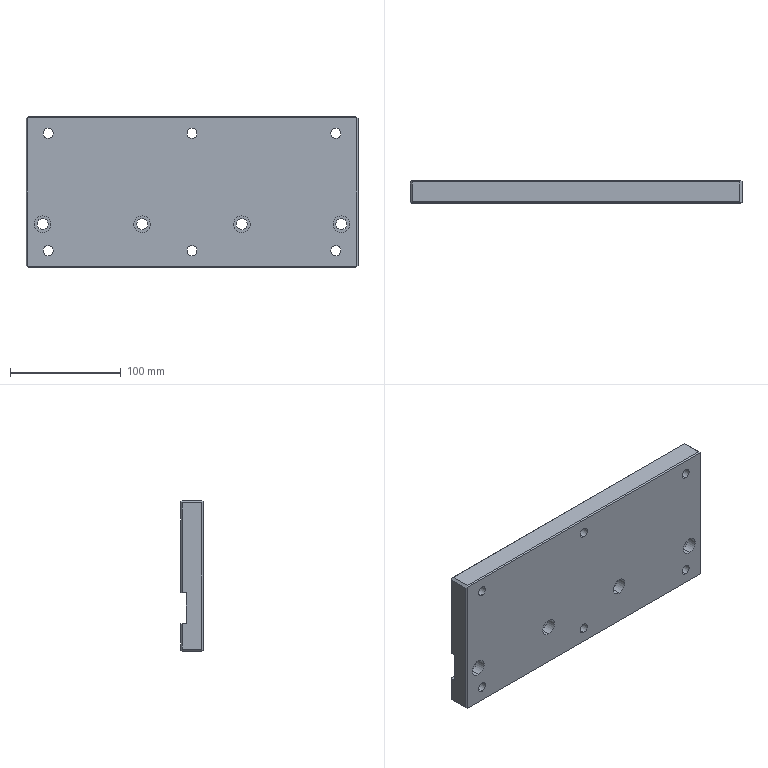Part | STEP file | 10000020450swp000-1 | 1 solid | 74 faces | box 300 x 20 x 136 mm | volume 751021 mm3 | cylinder 40 | plane 34 | commonest cylinder face diameters 15 x20 9 x12 10 x8